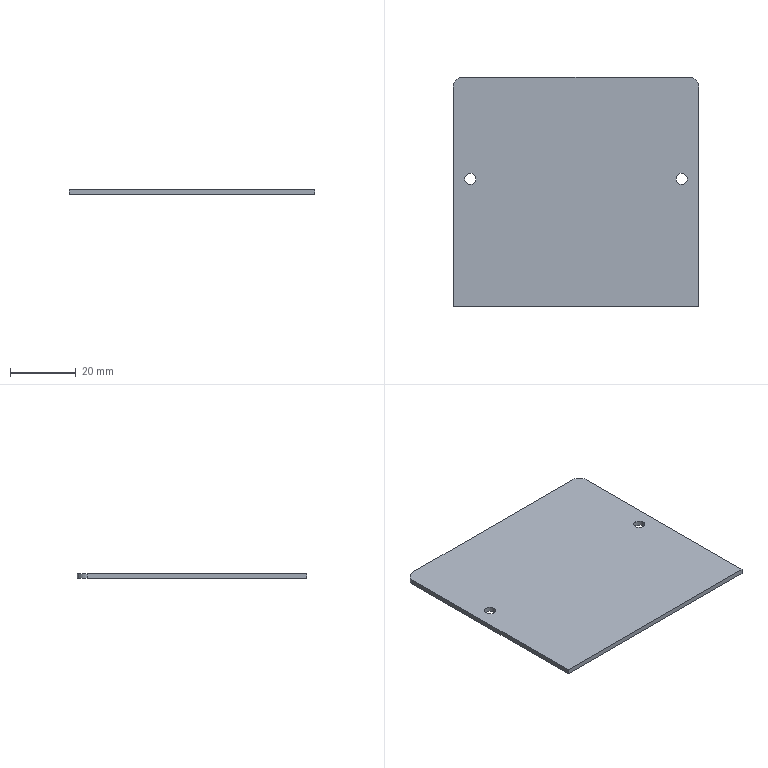Part | NX | features BREP 1 | 1 solid | 10 faces | box 75 x 70 x 1.5 mm | volume 7842 mm3 | plane 6 | cylinder 4 | commonest cylinder face diameters 3.4 x2 6 x2
STEP:
#1=CARTESIAN_POINT('',(33.95,4.,1.5));
#2=VERTEX_POINT('',#1);
#3=CARTESIAN_POINT('',(32.25,4.,1.5));
#4=DIRECTION('',(0.,0.,1.));
#5=DIRECTION('',(1.,0.,0.));
#6=AXIS2_PLACEMENT_3D('',#3,#4,#5);
#7=CIRCLE('',#6,1.7);
#8=EDGE_CURVE('',#2,#2,#7,.T.);
#9=ORIENTED_EDGE('',*,*,#8,.T.);
#10=EDGE_LOOP('',(#9));
#11=FACE_BOUND('',#10,.T.);
#12=CARTESIAN_POINT('',(33.95,4.,0.));
#13=VERTEX_POINT('',#12);
#14=CARTESIAN_POINT('',(32.25,4.,0.));
#15=DIRECTION('',(0.,0.,1.));
#16=DIRECTION('',(1.,0.,0.));
#17=AXIS2_PLACEMENT_3D('',#14,#15,#16);
#18=CIRCLE('',#17,1.7);
#19=EDGE_CURVE('',#13,#13,#18,.T.);
#20=ORIENTED_EDGE('',*,*,#19,.F.);
#21=EDGE_LOOP('',(#20));
#22=FACE_BOUND('',#21,.T.);
#23=CARTESIAN_POINT('',(32.25,4.,1.5));
#24=DIRECTION('',(0.,0.,1.));
#25=DIRECTION('',(1.,0.,0.));
#26=AXIS2_PLACEMENT_3D('',#23,#24,#25);
#27=CYLINDRICAL_SURFACE('',#26,1.7);
#28=ADVANCED_FACE('',(#11,#22),#27,.F.);
#29=CARTESIAN_POINT('',(-30.55,4.,1.5));
#30=VERTEX_POINT('',#29);
#31=CARTESIAN_POINT('',(-32.25,4.,1.5));
#32=DIRECTION('',(0.,0.,1.));
#33=DIRECTION('',(1.,0.,0.));
#34=AXIS2_PLACEMENT_3D('',#31,#32,#33);
#35=CIRCLE('',#34,1.7);
#36=EDGE_CURVE('',#30,#30,#35,.T.);
#37=ORIENTED_EDGE('',*,*,#36,.T.);
#38=EDGE_LOOP('',(#37));
#39=FACE_BOUND('',#38,.T.);
#40=CARTESIAN_POINT('',(-30.55,4.,0.));
#41=VERTEX_POINT('',#40);
#42=CARTESIAN_POINT('',(-32.25,4.,0.));
#43=DIRECTION('',(0.,0.,1.));
#44=DIRECTION('',(1.,0.,0.));
#45=AXIS2_PLACEMENT_3D('',#42,#43,#44);
#46=CIRCLE('',#45,1.7);
#47=EDGE_CURVE('',#41,#41,#46,.T.);
#48=ORIENTED_EDGE('',*,*,#47,.F.);
#49=EDGE_LOOP('',(#48));
#50=FACE_BOUND('',#49,.T.);
#51=CARTESIAN_POINT('',(-32.25,4.,1.5));
#52=DIRECTION('',(0.,0.,1.));
#53=DIRECTION('',(1.,0.,0.));
#54=AXIS2_PLACEMENT_3D('',#51,#52,#53);
#55=CYLINDRICAL_SURFACE('',#54,1.7);
#56=ADVANCED_FACE('',(#39,#50),#55,.F.);
#57=CARTESIAN_POINT('',(37.5,-35.,0.));
#58=VERTEX_POINT('',#57);
#59=CARTESIAN_POINT('',(37.5,32.,0.));
#60=VERTEX_POINT('',#59);
#61=CARTESIAN_POINT('',(37.5,35.,0.));
#62=DIRECTION('',(0.,1.,0.));
#63=VECTOR('',#62,1000.);
#64=LINE('',#61,#63);
#65=EDGE_CURVE('',#58,#60,#64,.T.);
#66=ORIENTED_EDGE('',*,*,#65,.T.);
#67=CARTESIAN_POINT('',(37.5,32.,1.5));
#68=VERTEX_POINT('',#67);
#69=CARTESIAN_POINT('',(37.5,32.,1.5));
#70=DIRECTION('',(0.,0.,1.));
#71=VECTOR('',#70,1000.);
#72=LINE('',#69,#71);
#73=EDGE_CURVE('',#60,#68,#72,.T.);
#74=ORIENTED_EDGE('',*,*,#73,.T.);
#75=CARTESIAN_POINT('',(37.5,-35.,1.5));
#76=VERTEX_POINT('',#75);
#77=CARTESIAN_POINT('',(37.5,35.,1.5));
#78=DIRECTION('',(0.,1.,0.));
#79=VECTOR('',#78,1000.);
#80=LINE('',#77,#79);
#81=EDGE_CURVE('',#76,#68,#80,.T.);
#82=ORIENTED_EDGE('',*,*,#81,.F.);
#83=CARTESIAN_POINT('',(37.5,-35.,1.5));
#84=DIRECTION('',(0.,0.,-1.));
#85=VECTOR('',#84,1000.);
#86=LINE('',#83,#85);
#87=EDGE_CURVE('',#76,#58,#86,.T.);
#88=ORIENTED_EDGE('',*,*,#87,.T.);
#89=EDGE_LOOP('',(#66,#74,#82,#88));
#90=FACE_BOUND('',#89,.T.);
#91=CARTESIAN_POINT('',(37.5,35.,1.5));
#92=DIRECTION('',(-1.,0.,0.));
#93=DIRECTION('',(0.,-1.,0.));
#94=AXIS2_PLACEMENT_3D('',#91,#92,#93);
#95=PLANE('',#94);
#96=ADVANCED_FACE('',(#90),#95,.F.);
#97=CARTESIAN_POINT('',(34.5,35.,0.));
#98=VERTEX_POINT('',#97);
#99=CARTESIAN_POINT('',(-34.5,35.,0.));
#100=VERTEX_POINT('',#99);
#101=CARTESIAN_POINT('',(-37.5,35.,0.));
#102=DIRECTION('',(-1.,0.,0.));
#103=VECTOR('',#102,1000.);
#104=LINE('',#101,#103);
#105=EDGE_CURVE('',#98,#100,#104,.T.);
#106=ORIENTED_EDGE('',*,*,#105,.T.);
#107=CARTESIAN_POINT('',(-34.5,35.,1.5));
#108=VERTEX_POINT('',#107);
#109=CARTESIAN_POINT('',(-34.5,35.,1.5));
#110=DIRECTION('',(0.,0.,1.));
#111=VECTOR('',#110,1000.);
#112=LINE('',#109,#111);
#113=EDGE_CURVE('',#100,#108,#112,.T.);
#114=ORIENTED_EDGE('',*,*,#113,.T.);
#115=CARTESIAN_POINT('',(34.5,35.,1.5));
#116=VERTEX_POINT('',#115);
#117=CARTESIAN_POINT('',(-37.5,35.,1.5));
#118=DIRECTION('',(-1.,0.,0.));
#119=VECTOR('',#118,1000.);
#120=LINE('',#117,#119);
#121=EDGE_CURVE('',#116,#108,#120,.T.);
#122=ORIENTED_EDGE('',*,*,#121,.F.);
#123=CARTESIAN_POINT('',(34.5,35.,1.5));
#124=DIRECTION('',(0.,0.,-1.));
#125=VECTOR('',#124,1000.);
#126=LINE('',#123,#125);
#127=EDGE_CURVE('',#116,#98,#126,.T.);
#128=ORIENTED_EDGE('',*,*,#127,.T.);
#129=EDGE_LOOP('',(#106,#114,#122,#128));
#130=FACE_BOUND('',#129,.T.);
#131=CARTESIAN_POINT('',(-37.5,35.,1.5));
#132=DIRECTION('',(0.,-1.,0.));
#133=DIRECTION('',(0.,0.,-1.));
#134=AXIS2_PLACEMENT_3D('',#131,#132,#133);
#135=PLANE('',#134);
#136=ADVANCED_FACE('',(#130),#135,.F.);
#137=CARTESIAN_POINT('',(-37.5,32.,1.5));
#138=VERTEX_POINT('',#137);
#139=CARTESIAN_POINT('',(-37.5,-35.,1.5));
#140=VERTEX_POINT('',#139);
#141=CARTESIAN_POINT('',(-37.5,35.,1.5));
#142=DIRECTION('',(0.,-1.,0.));
#143=VECTOR('',#142,1000.);
#144=LINE('',#141,#143);
#145=EDGE_CURVE('',#138,#140,#144,.T.);
#146=ORIENTED_EDGE('',*,*,#145,.F.);
#147=CARTESIAN_POINT('',(-37.5,32.,0.));
#148=VERTEX_POINT('',#147);
#149=CARTESIAN_POINT('',(-37.5,32.,1.5));
#150=DIRECTION('',(0.,0.,-1.));
#151=VECTOR('',#150,1000.);
#152=LINE('',#149,#151);
#153=EDGE_CURVE('',#138,#148,#152,.T.);
#154=ORIENTED_EDGE('',*,*,#153,.T.);
#155=CARTESIAN_POINT('',(-37.5,-35.,0.));
#156=VERTEX_POINT('',#155);
#157=CARTESIAN_POINT('',(-37.5,35.,0.));
#158=DIRECTION('',(0.,-1.,0.));
#159=VECTOR('',#158,1000.);
#160=LINE('',#157,#159);
#161=EDGE_CURVE('',#148,#156,#160,.T.);
#162=ORIENTED_EDGE('',*,*,#161,.T.);
#163=CARTESIAN_POINT('',(-37.5,-35.,1.5));
#164=DIRECTION('',(0.,0.,-1.));
#165=VECTOR('',#164,1000.);
#166=LINE('',#163,#165);
#167=EDGE_CURVE('',#140,#156,#166,.T.);
#168=ORIENTED_EDGE('',*,*,#167,.F.);
#169=EDGE_LOOP('',(#146,#154,#162,#168));
#170=FACE_BOUND('',#169,.T.);
#171=CARTESIAN_POINT('',(-37.5,35.,1.5));
#172=DIRECTION('',(1.,0.,0.));
#173=DIRECTION('',(0.,1.,0.));
#174=AXIS2_PLACEMENT_3D('',#171,#172,#173);
#175=PLANE('',#174);
#176=ADVANCED_FACE('',(#170),#175,.F.);
#177=CARTESIAN_POINT('',(-37.5,-35.,0.));
#178=DIRECTION('',(1.,0.,0.));
#179=VECTOR('',#178,1000.);
#180=LINE('',#177,#179);
#181=EDGE_CURVE('',#156,#58,#180,.T.);
#182=ORIENTED_EDGE('',*,*,#181,.T.);
#183=ORIENTED_EDGE('',*,*,#87,.F.);
#184=CARTESIAN_POINT('',(-37.5,-35.,1.5));
#185=DIRECTION('',(1.,0.,0.));
#186=VECTOR('',#185,1000.);
#187=LINE('',#184,#186);
#188=EDGE_CURVE('',#140,#76,#187,.T.);
#189=ORIENTED_EDGE('',*,*,#188,.F.);
#190=ORIENTED_EDGE('',*,*,#167,.T.);
#191=EDGE_LOOP('',(#182,#183,#189,#190));
#192=FACE_BOUND('',#191,.T.);
#193=CARTESIAN_POINT('',(-37.5,-35.,1.5));
#194=DIRECTION('',(0.,1.,0.));
#195=DIRECTION('',(0.,0.,1.));
#196=AXIS2_PLACEMENT_3D('',#193,#194,#195);
#197=PLANE('',#196);
#198=ADVANCED_FACE('',(#192),#197,.F.);
#199=ORIENTED_EDGE('',*,*,#8,.F.);
#200=EDGE_LOOP('',(#199));
#201=FACE_BOUND('',#200,.T.);
#202=ORIENTED_EDGE('',*,*,#36,.F.);
#203=EDGE_LOOP('',(#202));
#204=FACE_BOUND('',#203,.T.);
#205=ORIENTED_EDGE('',*,*,#121,.T.);
#206=CARTESIAN_POINT('',(-34.5,32.,1.5));
#207=DIRECTION('',(0.,0.,1.));
#208=DIRECTION('',(1.,0.,0.));
#209=AXIS2_PLACEMENT_3D('',#206,#207,#208);
#210=CIRCLE('',#209,3.);
#211=EDGE_CURVE('',#108,#138,#210,.T.);
#212=ORIENTED_EDGE('',*,*,#211,.T.);
#213=ORIENTED_EDGE('',*,*,#145,.T.);
#214=ORIENTED_EDGE('',*,*,#188,.T.);
#215=ORIENTED_EDGE('',*,*,#81,.T.);
#216=CARTESIAN_POINT('',(34.5,32.,1.5));
#217=DIRECTION('',(0.,0.,1.));
#218=DIRECTION('',(1.,0.,0.));
#219=AXIS2_PLACEMENT_3D('',#216,#217,#218);
#220=CIRCLE('',#219,3.);
#221=EDGE_CURVE('',#68,#116,#220,.T.);
#222=ORIENTED_EDGE('',*,*,#221,.T.);
#223=EDGE_LOOP('',(#205,#212,#213,#214,#215,#222));
#224=FACE_BOUND('',#223,.T.);
#225=CARTESIAN_POINT('',(0.,0.,1.5));
#226=DIRECTION('',(0.,0.,1.));
#227=DIRECTION('',(1.,0.,0.));
#228=AXIS2_PLACEMENT_3D('',#225,#226,#227);
#229=PLANE('',#228);
#230=ADVANCED_FACE('',(#201,#204,#224),#229,.T.);
#231=ORIENTED_EDGE('',*,*,#19,.T.);
#232=EDGE_LOOP('',(#231));
#233=FACE_BOUND('',#232,.T.);
#234=ORIENTED_EDGE('',*,*,#47,.T.);
#235=EDGE_LOOP('',(#234));
#236=FACE_BOUND('',#235,.T.);
#237=ORIENTED_EDGE('',*,*,#161,.F.);
#238=CARTESIAN_POINT('',(-34.5,32.,0.));
#239=DIRECTION('',(0.,0.,-1.));
#240=DIRECTION('',(1.,0.,0.));
#241=AXIS2_PLACEMENT_3D('',#238,#239,#240);
#242=CIRCLE('',#241,3.);
#243=EDGE_CURVE('',#148,#100,#242,.T.);
#244=ORIENTED_EDGE('',*,*,#243,.T.);
#245=ORIENTED_EDGE('',*,*,#105,.F.);
#246=CARTESIAN_POINT('',(34.5,32.,0.));
#247=DIRECTION('',(0.,0.,-1.));
#248=DIRECTION('',(1.,0.,0.));
#249=AXIS2_PLACEMENT_3D('',#246,#247,#248);
#250=CIRCLE('',#249,3.);
#251=EDGE_CURVE('',#98,#60,#250,.T.);
#252=ORIENTED_EDGE('',*,*,#251,.T.);
#253=ORIENTED_EDGE('',*,*,#65,.F.);
#254=ORIENTED_EDGE('',*,*,#181,.F.);
#255=EDGE_LOOP('',(#237,#244,#245,#252,#253,#254));
#256=FACE_BOUND('',#255,.T.);
#257=CARTESIAN_POINT('',(0.,0.,0.));
#258=DIRECTION('',(0.,0.,1.));
#259=DIRECTION('',(1.,0.,0.));
#260=AXIS2_PLACEMENT_3D('',#257,#258,#259);
#261=PLANE('',#260);
#262=ADVANCED_FACE('',(#233,#236,#256),#261,.F.);
#263=ORIENTED_EDGE('',*,*,#211,.F.);
#264=ORIENTED_EDGE('',*,*,#113,.F.);
#265=ORIENTED_EDGE('',*,*,#243,.F.);
#266=ORIENTED_EDGE('',*,*,#153,.F.);
#267=EDGE_LOOP('',(#263,#264,#265,#266));
#268=FACE_BOUND('',#267,.T.);
#269=CARTESIAN_POINT('',(-34.5,32.,1.5));
#270=DIRECTION('',(0.,0.,-1.));
#271=DIRECTION('',(-1.,0.,0.));
#272=AXIS2_PLACEMENT_3D('',#269,#270,#271);
#273=CYLINDRICAL_SURFACE('',#272,3.);
#274=ADVANCED_FACE('',(#268),#273,.T.);
#275=ORIENTED_EDGE('',*,*,#221,.F.);
#276=ORIENTED_EDGE('',*,*,#73,.F.);
#277=ORIENTED_EDGE('',*,*,#251,.F.);
#278=ORIENTED_EDGE('',*,*,#127,.F.);
#279=EDGE_LOOP('',(#275,#276,#277,#278));
#280=FACE_BOUND('',#279,.T.);
#281=CARTESIAN_POINT('',(34.5,32.,1.5));
#282=DIRECTION('',(0.,0.,-1.));
#283=DIRECTION('',(-1.,0.,0.));
#284=AXIS2_PLACEMENT_3D('',#281,#282,#283);
#285=CYLINDRICAL_SURFACE('',#284,3.);
#286=ADVANCED_FACE('',(#280),#285,.T.);
#287=CLOSED_SHELL('',(#28,#56,#96,#136,#176,#198,#230,#262,#274,#286));
#288=MANIFOLD_SOLID_BREP('',#287);
#289=(LENGTH_UNIT()NAMED_UNIT(*)SI_UNIT(.MILLI.,.METRE.));
#290=UNCERTAINTY_MEASURE_WITH_UNIT(LENGTH_MEASURE(0.00001),#289,'','');
#291=(NAMED_UNIT(*)PLANE_ANGLE_UNIT()SI_UNIT($,.RADIAN.));
#292=(NAMED_UNIT(*)SI_UNIT($,.STERADIAN.)SOLID_ANGLE_UNIT());
#293=(GEOMETRIC_REPRESENTATION_CONTEXT(3)GLOBAL_UNCERTAINTY_ASSIGNED_CONTEXT((#290))GLOBAL_UNIT_ASSIGNED_CONTEXT((#289,#291,#292))REPRESENTATION_CONTEXT('',''));
#294=ADVANCED_BREP_SHAPE_REPRESENTATION('',(#288),#293);